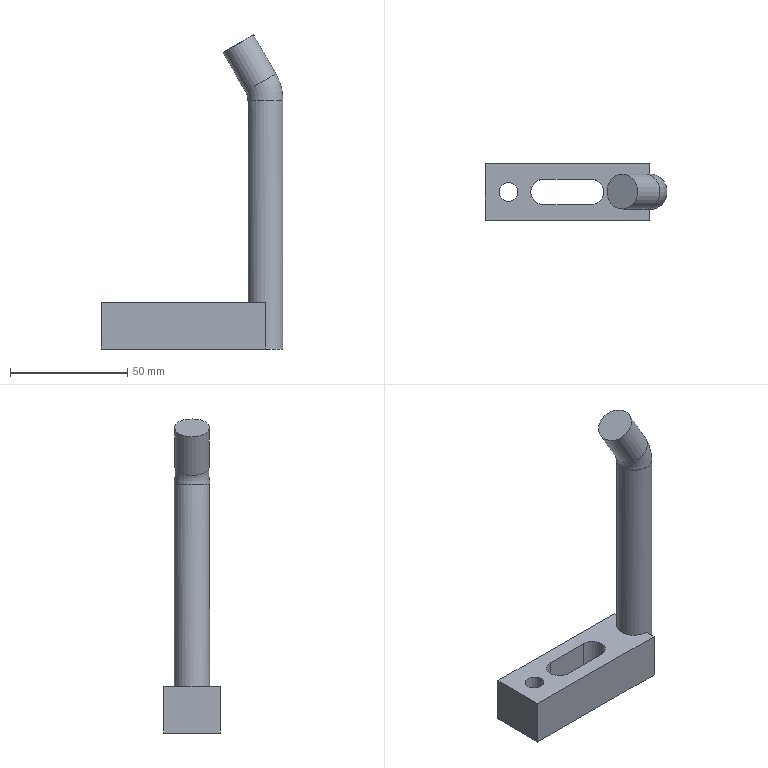Part | NX | features solid 2 | 1 solid | 16 faces | box 77.5 x 24 x 133.75 mm | volume 48014 mm3 | plane 10 | cylinder 5 | torus 1 | commonest cylinder face diameters 11 x2 15 x2 8 x1
STEP:
#1=CARTESIAN_POINT('',(-693.,-167.5,-90.));
#2=VERTEX_POINT('',#1);
#3=CARTESIAN_POINT('',(-693.,-167.5,-70.));
#4=VERTEX_POINT('',#3);
#5=CARTESIAN_POINT('',(-693.,-167.5,15.981));
#6=DIRECTION('',(0.,0.,-1.));
#7=VECTOR('',#6,1000.);
#8=LINE('',#5,#7);
#9=EDGE_CURVE('',#2,#4,#8,.F.);
#10=ORIENTED_EDGE('',*,*,#9,.T.);
#11=CARTESIAN_POINT('',(-693.,-172.,-70.));
#12=VERTEX_POINT('',#11);
#13=CARTESIAN_POINT('',(-693.,-148.,-70.));
#14=DIRECTION('',(0.,-1.,0.));
#15=VECTOR('',#14,1000.);
#16=LINE('',#13,#15);
#17=EDGE_CURVE('',#4,#12,#16,.T.);
#18=ORIENTED_EDGE('',*,*,#17,.T.);
#19=CARTESIAN_POINT('',(-693.,-172.,-90.));
#20=VERTEX_POINT('',#19);
#21=CARTESIAN_POINT('',(-693.,-172.,-70.));
#22=DIRECTION('',(0.,0.,-1.));
#23=VECTOR('',#22,1000.);
#24=LINE('',#21,#23);
#25=EDGE_CURVE('',#12,#20,#24,.T.);
#26=ORIENTED_EDGE('',*,*,#25,.T.);
#27=CARTESIAN_POINT('',(-693.,-148.,-90.));
#28=DIRECTION('',(0.,-1.,0.));
#29=VECTOR('',#28,1000.);
#30=LINE('',#27,#29);
#31=EDGE_CURVE('',#2,#20,#30,.T.);
#32=ORIENTED_EDGE('',*,*,#31,.F.);
#33=EDGE_LOOP('',(#10,#18,#26,#32));
#34=FACE_BOUND('',#33,.T.);
#35=CARTESIAN_POINT('',(-693.,-148.,-70.));
#36=DIRECTION('',(-1.,0.,0.));
#37=DIRECTION('',(0.,0.,-1.));
#38=AXIS2_PLACEMENT_3D('',#35,#36,#37);
#39=PLANE('',#38);
#40=ADVANCED_FACE('',(#34),#39,.F.);
#41=CARTESIAN_POINT('',(-693.,-152.5,-70.));
#42=VERTEX_POINT('',#41);
#43=CARTESIAN_POINT('',(-693.,-152.5,-90.));
#44=VERTEX_POINT('',#43);
#45=CARTESIAN_POINT('',(-693.,-152.5,15.981));
#46=DIRECTION('',(0.,0.,-1.));
#47=VECTOR('',#46,1000.);
#48=LINE('',#45,#47);
#49=EDGE_CURVE('',#42,#44,#48,.T.);
#50=ORIENTED_EDGE('',*,*,#49,.T.);
#51=CARTESIAN_POINT('',(-693.,-148.,-90.));
#52=VERTEX_POINT('',#51);
#53=CARTESIAN_POINT('',(-693.,-148.,-90.));
#54=DIRECTION('',(0.,-1.,0.));
#55=VECTOR('',#54,1000.);
#56=LINE('',#53,#55);
#57=EDGE_CURVE('',#52,#44,#56,.T.);
#58=ORIENTED_EDGE('',*,*,#57,.F.);
#59=CARTESIAN_POINT('',(-693.,-148.,-70.));
#60=VERTEX_POINT('',#59);
#61=CARTESIAN_POINT('',(-693.,-148.,-70.));
#62=DIRECTION('',(0.,0.,-1.));
#63=VECTOR('',#62,1000.);
#64=LINE('',#61,#63);
#65=EDGE_CURVE('',#60,#52,#64,.T.);
#66=ORIENTED_EDGE('',*,*,#65,.F.);
#67=CARTESIAN_POINT('',(-693.,-148.,-70.));
#68=DIRECTION('',(0.,-1.,0.));
#69=VECTOR('',#68,1000.);
#70=LINE('',#67,#69);
#71=EDGE_CURVE('',#60,#42,#70,.T.);
#72=ORIENTED_EDGE('',*,*,#71,.T.);
#73=EDGE_LOOP('',(#50,#58,#66,#72));
#74=FACE_BOUND('',#73,.T.);
#75=CARTESIAN_POINT('',(-693.,-148.,-70.));
#76=DIRECTION('',(-1.,0.,0.));
#77=DIRECTION('',(0.,0.,-1.));
#78=AXIS2_PLACEMENT_3D('',#75,#76,#77);
#79=PLANE('',#78);
#80=ADVANCED_FACE('',(#74),#79,.F.);
#81=CARTESIAN_POINT('',(-718.,-154.5,-70.));
#82=VERTEX_POINT('',#81);
#83=CARTESIAN_POINT('',(-738.,-154.5,-70.));
#84=VERTEX_POINT('',#83);
#85=CARTESIAN_POINT('',(-728.,-154.5,-70.));
#86=DIRECTION('',(-1.,0.,0.));
#87=VECTOR('',#86,1000.);
#88=LINE('',#85,#87);
#89=EDGE_CURVE('',#82,#84,#88,.T.);
#90=ORIENTED_EDGE('',*,*,#89,.F.);
#91=CARTESIAN_POINT('',(-718.,-165.5,-70.));
#92=VERTEX_POINT('',#91);
#93=CARTESIAN_POINT('',(-718.,-160.,-70.));
#94=DIRECTION('',(0.,0.,-1.));
#95=DIRECTION('',(-1.,0.,0.));
#96=AXIS2_PLACEMENT_3D('',#93,#94,#95);
#97=CIRCLE('',#96,5.5);
#98=EDGE_CURVE('',#82,#92,#97,.T.);
#99=ORIENTED_EDGE('',*,*,#98,.T.);
#100=CARTESIAN_POINT('',(-738.,-165.5,-70.));
#101=VERTEX_POINT('',#100);
#102=CARTESIAN_POINT('',(-728.,-165.5,-70.));
#103=DIRECTION('',(-1.,0.,0.));
#104=VECTOR('',#103,1000.);
#105=LINE('',#102,#104);
#106=EDGE_CURVE('',#92,#101,#105,.T.);
#107=ORIENTED_EDGE('',*,*,#106,.T.);
#108=CARTESIAN_POINT('',(-738.,-160.,-70.));
#109=DIRECTION('',(0.,0.,-1.));
#110=DIRECTION('',(-1.,0.,0.));
#111=AXIS2_PLACEMENT_3D('',#108,#109,#110);
#112=CIRCLE('',#111,5.5);
#113=EDGE_CURVE('',#101,#84,#112,.T.);
#114=ORIENTED_EDGE('',*,*,#113,.T.);
#115=EDGE_LOOP('',(#90,#99,#107,#114));
#116=FACE_BOUND('',#115,.T.);
#117=CARTESIAN_POINT('',(-749.,-160.,-70.));
#118=VERTEX_POINT('',#117);
#119=CARTESIAN_POINT('',(-753.,-160.,-70.));
#120=DIRECTION('',(0.,0.,1.));
#121=DIRECTION('',(1.,0.,0.));
#122=AXIS2_PLACEMENT_3D('',#119,#120,#121);
#123=CIRCLE('',#122,4.);
#124=EDGE_CURVE('',#118,#118,#123,.T.);
#125=ORIENTED_EDGE('',*,*,#124,.F.);
#126=EDGE_LOOP('',(#125));
#127=FACE_BOUND('',#126,.T.);
#128=ORIENTED_EDGE('',*,*,#71,.F.);
#129=CARTESIAN_POINT('',(-763.,-148.,-70.));
#130=VERTEX_POINT('',#129);
#131=CARTESIAN_POINT('',(-763.,-148.,-70.));
#132=DIRECTION('',(1.,0.,0.));
#133=VECTOR('',#132,1000.);
#134=LINE('',#131,#133);
#135=EDGE_CURVE('',#130,#60,#134,.T.);
#136=ORIENTED_EDGE('',*,*,#135,.F.);
#137=CARTESIAN_POINT('',(-763.,-172.,-70.));
#138=VERTEX_POINT('',#137);
#139=CARTESIAN_POINT('',(-763.,-172.,-70.));
#140=DIRECTION('',(0.,1.,0.));
#141=VECTOR('',#140,1000.);
#142=LINE('',#139,#141);
#143=EDGE_CURVE('',#138,#130,#142,.T.);
#144=ORIENTED_EDGE('',*,*,#143,.F.);
#145=CARTESIAN_POINT('',(-693.,-172.,-70.));
#146=DIRECTION('',(-1.,0.,0.));
#147=VECTOR('',#146,1000.);
#148=LINE('',#145,#147);
#149=EDGE_CURVE('',#12,#138,#148,.T.);
#150=ORIENTED_EDGE('',*,*,#149,.F.);
#151=ORIENTED_EDGE('',*,*,#17,.F.);
#152=CARTESIAN_POINT('',(-693.,-160.,-70.));
#153=DIRECTION('',(0.,0.,-1.));
#154=DIRECTION('',(-1.,0.,0.));
#155=AXIS2_PLACEMENT_3D('',#152,#153,#154);
#156=CIRCLE('',#155,7.5);
#157=EDGE_CURVE('',#42,#4,#156,.F.);
#158=ORIENTED_EDGE('',*,*,#157,.F.);
#159=EDGE_LOOP('',(#128,#136,#144,#150,#151,#158));
#160=FACE_BOUND('',#159,.T.);
#161=CARTESIAN_POINT('',(-763.,-148.,-70.));
#162=DIRECTION('',(0.,0.,1.));
#163=DIRECTION('',(-1.,0.,0.));
#164=AXIS2_PLACEMENT_3D('',#161,#162,#163);
#165=PLANE('',#164);
#166=ADVANCED_FACE('',(#116,#127,#160),#165,.T.);
#167=CARTESIAN_POINT('',(-763.,-172.,-90.));
#168=VERTEX_POINT('',#167);
#169=CARTESIAN_POINT('',(-763.,-148.,-90.));
#170=VERTEX_POINT('',#169);
#171=CARTESIAN_POINT('',(-763.,-172.,-90.));
#172=DIRECTION('',(0.,1.,0.));
#173=VECTOR('',#172,1000.);
#174=LINE('',#171,#173);
#175=EDGE_CURVE('',#168,#170,#174,.T.);
#176=ORIENTED_EDGE('',*,*,#175,.F.);
#177=CARTESIAN_POINT('',(-763.,-172.,-70.));
#178=DIRECTION('',(0.,0.,-1.));
#179=VECTOR('',#178,1000.);
#180=LINE('',#177,#179);
#181=EDGE_CURVE('',#138,#168,#180,.T.);
#182=ORIENTED_EDGE('',*,*,#181,.F.);
#183=ORIENTED_EDGE('',*,*,#143,.T.);
#184=CARTESIAN_POINT('',(-763.,-148.,-70.));
#185=DIRECTION('',(0.,0.,-1.));
#186=VECTOR('',#185,1000.);
#187=LINE('',#184,#186);
#188=EDGE_CURVE('',#130,#170,#187,.T.);
#189=ORIENTED_EDGE('',*,*,#188,.T.);
#190=EDGE_LOOP('',(#176,#182,#183,#189));
#191=FACE_BOUND('',#190,.T.);
#192=CARTESIAN_POINT('',(-763.,-172.,-70.));
#193=DIRECTION('',(1.,0.,0.));
#194=DIRECTION('',(0.,0.,1.));
#195=AXIS2_PLACEMENT_3D('',#192,#193,#194);
#196=PLANE('',#195);
#197=ADVANCED_FACE('',(#191),#196,.F.);
#198=CARTESIAN_POINT('',(-763.,-148.,-90.));
#199=DIRECTION('',(1.,0.,0.));
#200=VECTOR('',#199,1000.);
#201=LINE('',#198,#200);
#202=EDGE_CURVE('',#170,#52,#201,.T.);
#203=ORIENTED_EDGE('',*,*,#202,.F.);
#204=ORIENTED_EDGE('',*,*,#188,.F.);
#205=ORIENTED_EDGE('',*,*,#135,.T.);
#206=ORIENTED_EDGE('',*,*,#65,.T.);
#207=EDGE_LOOP('',(#203,#204,#205,#206));
#208=FACE_BOUND('',#207,.T.);
#209=CARTESIAN_POINT('',(-763.,-148.,-70.));
#210=DIRECTION('',(0.,-1.,0.));
#211=DIRECTION('',(-1.,0.,0.));
#212=AXIS2_PLACEMENT_3D('',#209,#210,#211);
#213=PLANE('',#212);
#214=ADVANCED_FACE('',(#208),#213,.F.);
#215=CARTESIAN_POINT('',(-693.,-172.,-90.));
#216=DIRECTION('',(-1.,0.,0.));
#217=VECTOR('',#216,1000.);
#218=LINE('',#215,#217);
#219=EDGE_CURVE('',#20,#168,#218,.T.);
#220=ORIENTED_EDGE('',*,*,#219,.F.);
#221=ORIENTED_EDGE('',*,*,#25,.F.);
#222=ORIENTED_EDGE('',*,*,#149,.T.);
#223=ORIENTED_EDGE('',*,*,#181,.T.);
#224=EDGE_LOOP('',(#220,#221,#222,#223));
#225=FACE_BOUND('',#224,.T.);
#226=CARTESIAN_POINT('',(-693.,-172.,-70.));
#227=DIRECTION('',(0.,1.,0.));
#228=DIRECTION('',(1.,0.,0.));
#229=AXIS2_PLACEMENT_3D('',#226,#227,#228);
#230=PLANE('',#229);
#231=ADVANCED_FACE('',(#225),#230,.F.);
#232=ORIENTED_EDGE('',*,*,#31,.T.);
#233=ORIENTED_EDGE('',*,*,#219,.T.);
#234=ORIENTED_EDGE('',*,*,#175,.T.);
#235=ORIENTED_EDGE('',*,*,#202,.T.);
#236=ORIENTED_EDGE('',*,*,#57,.T.);
#237=CARTESIAN_POINT('',(-693.,-160.,-90.));
#238=DIRECTION('',(0.,0.,-1.));
#239=DIRECTION('',(-1.,0.,0.));
#240=AXIS2_PLACEMENT_3D('',#237,#238,#239);
#241=CIRCLE('',#240,7.5);
#242=EDGE_CURVE('',#44,#2,#241,.T.);
#243=ORIENTED_EDGE('',*,*,#242,.T.);
#244=EDGE_LOOP('',(#232,#233,#234,#235,#236,#243));
#245=FACE_BOUND('',#244,.T.);
#246=CARTESIAN_POINT('',(-738.,-165.5,-90.));
#247=VERTEX_POINT('',#246);
#248=CARTESIAN_POINT('',(-738.,-154.5,-90.));
#249=VERTEX_POINT('',#248);
#250=CARTESIAN_POINT('',(-738.,-160.,-90.));
#251=DIRECTION('',(0.,0.,-1.));
#252=DIRECTION('',(-1.,0.,0.));
#253=AXIS2_PLACEMENT_3D('',#250,#251,#252);
#254=CIRCLE('',#253,5.5);
#255=EDGE_CURVE('',#247,#249,#254,.T.);
#256=ORIENTED_EDGE('',*,*,#255,.F.);
#257=CARTESIAN_POINT('',(-718.,-165.5,-90.));
#258=VERTEX_POINT('',#257);
#259=CARTESIAN_POINT('',(-718.,-165.5,-90.));
#260=DIRECTION('',(-1.,0.,0.));
#261=VECTOR('',#260,1000.);
#262=LINE('',#259,#261);
#263=EDGE_CURVE('',#258,#247,#262,.T.);
#264=ORIENTED_EDGE('',*,*,#263,.F.);
#265=CARTESIAN_POINT('',(-718.,-154.5,-90.));
#266=VERTEX_POINT('',#265);
#267=CARTESIAN_POINT('',(-718.,-160.,-90.));
#268=DIRECTION('',(0.,0.,-1.));
#269=DIRECTION('',(-1.,0.,0.));
#270=AXIS2_PLACEMENT_3D('',#267,#268,#269);
#271=CIRCLE('',#270,5.5);
#272=EDGE_CURVE('',#266,#258,#271,.T.);
#273=ORIENTED_EDGE('',*,*,#272,.F.);
#274=CARTESIAN_POINT('',(-718.,-154.5,-90.));
#275=DIRECTION('',(-1.,0.,0.));
#276=VECTOR('',#275,1000.);
#277=LINE('',#274,#276);
#278=EDGE_CURVE('',#266,#249,#277,.T.);
#279=ORIENTED_EDGE('',*,*,#278,.T.);
#280=EDGE_LOOP('',(#256,#264,#273,#279));
#281=FACE_BOUND('',#280,.T.);
#282=CARTESIAN_POINT('',(-757.,-160.,-90.));
#283=VERTEX_POINT('',#282);
#284=CARTESIAN_POINT('',(-753.,-160.,-90.));
#285=DIRECTION('',(0.,0.,-1.));
#286=DIRECTION('',(-1.,0.,0.));
#287=AXIS2_PLACEMENT_3D('',#284,#285,#286);
#288=CIRCLE('',#287,4.);
#289=EDGE_CURVE('',#283,#283,#288,.T.);
#290=ORIENTED_EDGE('',*,*,#289,.F.);
#291=EDGE_LOOP('',(#290));
#292=FACE_BOUND('',#291,.T.);
#293=CARTESIAN_POINT('',(-763.,-148.,-90.));
#294=DIRECTION('',(0.,0.,1.));
#295=DIRECTION('',(-1.,0.,0.));
#296=AXIS2_PLACEMENT_3D('',#293,#294,#295);
#297=PLANE('',#296);
#298=ADVANCED_FACE('',(#245,#281,#292),#297,.F.);
#299=ORIENTED_EDGE('',*,*,#89,.T.);
#300=CARTESIAN_POINT('',(-738.,-154.5,-70.));
#301=DIRECTION('',(0.,0.,1.));
#302=VECTOR('',#301,1000.);
#303=LINE('',#300,#302);
#304=EDGE_CURVE('',#249,#84,#303,.T.);
#305=ORIENTED_EDGE('',*,*,#304,.F.);
#306=ORIENTED_EDGE('',*,*,#278,.F.);
#307=CARTESIAN_POINT('',(-718.,-154.5,-70.));
#308=DIRECTION('',(0.,0.,1.));
#309=VECTOR('',#308,1000.);
#310=LINE('',#307,#309);
#311=EDGE_CURVE('',#266,#82,#310,.T.);
#312=ORIENTED_EDGE('',*,*,#311,.T.);
#313=EDGE_LOOP('',(#299,#305,#306,#312));
#314=FACE_BOUND('',#313,.T.);
#315=CARTESIAN_POINT('',(-728.,-154.5,-70.));
#316=DIRECTION('',(0.,1.,0.));
#317=DIRECTION('',(0.,0.,1.));
#318=AXIS2_PLACEMENT_3D('',#315,#316,#317);
#319=PLANE('',#318);
#320=ADVANCED_FACE('',(#314),#319,.F.);
#321=ORIENTED_EDGE('',*,*,#98,.F.);
#322=ORIENTED_EDGE('',*,*,#311,.F.);
#323=ORIENTED_EDGE('',*,*,#272,.T.);
#324=CARTESIAN_POINT('',(-718.,-165.5,-70.));
#325=DIRECTION('',(0.,0.,1.));
#326=VECTOR('',#325,1000.);
#327=LINE('',#324,#326);
#328=EDGE_CURVE('',#258,#92,#327,.T.);
#329=ORIENTED_EDGE('',*,*,#328,.T.);
#330=EDGE_LOOP('',(#321,#322,#323,#329));
#331=FACE_BOUND('',#330,.T.);
#332=CARTESIAN_POINT('',(-718.,-160.,-70.));
#333=DIRECTION('',(0.,0.,1.));
#334=DIRECTION('',(-1.,0.,0.));
#335=AXIS2_PLACEMENT_3D('',#332,#333,#334);
#336=CYLINDRICAL_SURFACE('',#335,5.5);
#337=ADVANCED_FACE('',(#331),#336,.F.);
#338=ORIENTED_EDGE('',*,*,#106,.F.);
#339=ORIENTED_EDGE('',*,*,#328,.F.);
#340=ORIENTED_EDGE('',*,*,#263,.T.);
#341=CARTESIAN_POINT('',(-738.,-165.5,-70.));
#342=DIRECTION('',(0.,0.,1.));
#343=VECTOR('',#342,1000.);
#344=LINE('',#341,#343);
#345=EDGE_CURVE('',#247,#101,#344,.T.);
#346=ORIENTED_EDGE('',*,*,#345,.T.);
#347=EDGE_LOOP('',(#338,#339,#340,#346));
#348=FACE_BOUND('',#347,.T.);
#349=CARTESIAN_POINT('',(-728.,-165.5,-70.));
#350=DIRECTION('',(0.,-1.,0.));
#351=DIRECTION('',(0.,0.,-1.));
#352=AXIS2_PLACEMENT_3D('',#349,#350,#351);
#353=PLANE('',#352);
#354=ADVANCED_FACE('',(#348),#353,.F.);
#355=ORIENTED_EDGE('',*,*,#113,.F.);
#356=ORIENTED_EDGE('',*,*,#345,.F.);
#357=ORIENTED_EDGE('',*,*,#255,.T.);
#358=ORIENTED_EDGE('',*,*,#304,.T.);
#359=EDGE_LOOP('',(#355,#356,#357,#358));
#360=FACE_BOUND('',#359,.T.);
#361=CARTESIAN_POINT('',(-738.,-160.,-70.));
#362=DIRECTION('',(0.,0.,1.));
#363=DIRECTION('',(-1.,0.,0.));
#364=AXIS2_PLACEMENT_3D('',#361,#362,#363);
#365=CYLINDRICAL_SURFACE('',#364,5.5);
#366=ADVANCED_FACE('',(#360),#365,.F.);
#367=ORIENTED_EDGE('',*,*,#124,.T.);
#368=EDGE_LOOP('',(#367));
#369=FACE_BOUND('',#368,.T.);
#370=ORIENTED_EDGE('',*,*,#289,.T.);
#371=EDGE_LOOP('',(#370));
#372=FACE_BOUND('',#371,.T.);
#373=CARTESIAN_POINT('',(-753.,-160.,-70.));
#374=DIRECTION('',(0.,0.,-1.));
#375=DIRECTION('',(1.,0.,0.));
#376=AXIS2_PLACEMENT_3D('',#373,#374,#375);
#377=CYLINDRICAL_SURFACE('',#376,4.);
#378=ADVANCED_FACE('',(#369,#372),#377,.F.);
#379=CARTESIAN_POINT('',(-700.5,-160.,15.981));
#380=VERTEX_POINT('',#379);
#381=CARTESIAN_POINT('',(-693.,-160.,15.981));
#382=DIRECTION('',(0.,0.,-1.));
#383=DIRECTION('',(-1.,0.,0.));
#384=AXIS2_PLACEMENT_3D('',#381,#382,#383);
#385=CIRCLE('',#384,7.5);
#386=EDGE_CURVE('',#380,#380,#385,.T.);
#387=ORIENTED_EDGE('',*,*,#386,.T.);
#388=EDGE_LOOP('',(#387));
#389=FACE_BOUND('',#388,.T.);
#390=ORIENTED_EDGE('',*,*,#242,.F.);
#391=ORIENTED_EDGE('',*,*,#49,.F.);
#392=ORIENTED_EDGE('',*,*,#157,.T.);
#393=ORIENTED_EDGE('',*,*,#9,.F.);
#394=EDGE_LOOP('',(#390,#391,#392,#393));
#395=FACE_BOUND('',#394,.T.);
#396=CARTESIAN_POINT('',(-693.,-160.,15.981));
#397=DIRECTION('',(0.,0.,-1.));
#398=DIRECTION('',(1.,0.,0.));
#399=AXIS2_PLACEMENT_3D('',#396,#397,#398);
#400=CYLINDRICAL_SURFACE('',#399,7.5);
#401=ADVANCED_FACE('',(#389,#395),#400,.T.);
#402=CARTESIAN_POINT('',(-701.505,-160.,19.731));
#403=VERTEX_POINT('',#402);
#404=CARTESIAN_POINT('',(-695.01,-160.,23.481));
#405=DIRECTION('',(0.5,0.,-0.866));
#406=DIRECTION('',(-0.866,0.,-0.5));
#407=AXIS2_PLACEMENT_3D('',#404,#405,#406);
#408=CIRCLE('',#407,7.5);
#409=EDGE_CURVE('',#403,#403,#408,.T.);
#410=ORIENTED_EDGE('',*,*,#409,.F.);
#411=EDGE_LOOP('',(#410));
#412=FACE_BOUND('',#411,.T.);
#413=CARTESIAN_POINT('',(-711.042,-160.,36.25));
#414=VERTEX_POINT('',#413);
#415=CARTESIAN_POINT('',(-704.547,-160.,40.));
#416=DIRECTION('',(0.5,0.,-0.866));
#417=DIRECTION('',(-0.866,0.,-0.5));
#418=AXIS2_PLACEMENT_3D('',#415,#416,#417);
#419=CIRCLE('',#418,7.5);
#420=EDGE_CURVE('',#414,#414,#419,.T.);
#421=ORIENTED_EDGE('',*,*,#420,.T.);
#422=EDGE_LOOP('',(#421));
#423=FACE_BOUND('',#422,.T.);
#424=CARTESIAN_POINT('',(-695.01,-160.,23.481));
#425=DIRECTION('',(-0.5,0.,0.866));
#426=DIRECTION('',(-0.866,0.,-0.5));
#427=AXIS2_PLACEMENT_3D('',#424,#425,#426);
#428=CYLINDRICAL_SURFACE('',#427,7.5);
#429=ADVANCED_FACE('',(#412,#423),#428,.T.);
#430=ORIENTED_EDGE('',*,*,#386,.F.);
#431=EDGE_LOOP('',(#430));
#432=FACE_BOUND('',#431,.T.);
#433=ORIENTED_EDGE('',*,*,#409,.T.);
#434=EDGE_LOOP('',(#433));
#435=FACE_BOUND('',#434,.T.);
#436=CARTESIAN_POINT('',(-708.,-160.,15.981));
#437=DIRECTION('',(0.,1.,0.));
#438=DIRECTION('',(0.,0.,1.));
#439=AXIS2_PLACEMENT_3D('',#436,#437,#438);
#440=TOROIDAL_SURFACE('',#439,15.,7.5);
#441=ADVANCED_FACE('',(#432,#435),#440,.T.);
#442=ORIENTED_EDGE('',*,*,#420,.F.);
#443=EDGE_LOOP('',(#442));
#444=FACE_BOUND('',#443,.T.);
#445=CARTESIAN_POINT('',(-704.547,-160.,40.));
#446=DIRECTION('',(-0.5,0.,0.866));
#447=DIRECTION('',(-0.866,0.,-0.5));
#448=AXIS2_PLACEMENT_3D('',#445,#446,#447);
#449=PLANE('',#448);
#450=ADVANCED_FACE('',(#444),#449,.T.);
#451=CLOSED_SHELL('',(#40,#80,#166,#197,#214,#231,#298,#320,#337,#354,#366,#378,#401,#429,#441,#450));
#452=MANIFOLD_SOLID_BREP('',#451);
#453=(LENGTH_UNIT()NAMED_UNIT(*)SI_UNIT(.MILLI.,.METRE.));
#454=UNCERTAINTY_MEASURE_WITH_UNIT(LENGTH_MEASURE(0.00001),#453,'','');
#455=(NAMED_UNIT(*)PLANE_ANGLE_UNIT()SI_UNIT($,.RADIAN.));
#456=(NAMED_UNIT(*)SI_UNIT($,.STERADIAN.)SOLID_ANGLE_UNIT());
#457=(GEOMETRIC_REPRESENTATION_CONTEXT(3)GLOBAL_UNCERTAINTY_ASSIGNED_CONTEXT((#454))GLOBAL_UNIT_ASSIGNED_CONTEXT((#453,#455,#456))REPRESENTATION_CONTEXT('',''));
#458=ADVANCED_BREP_SHAPE_REPRESENTATION('',(#452),#457);